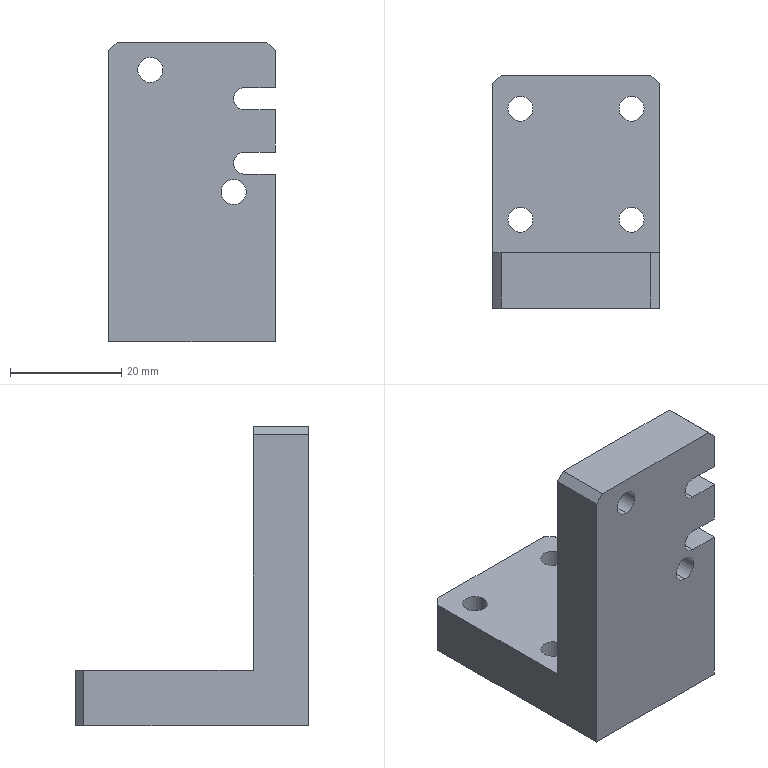Part | STEP file | PN_0057 Mount electronic clip finger cylinder mounting plate A | 1 solid | 34 faces | box 30 x 42 x 54 mm | volume 24235 mm3 | plane 18 | cylinder 16 | commonest cylinder face diameters 4.5 x12 4 x4